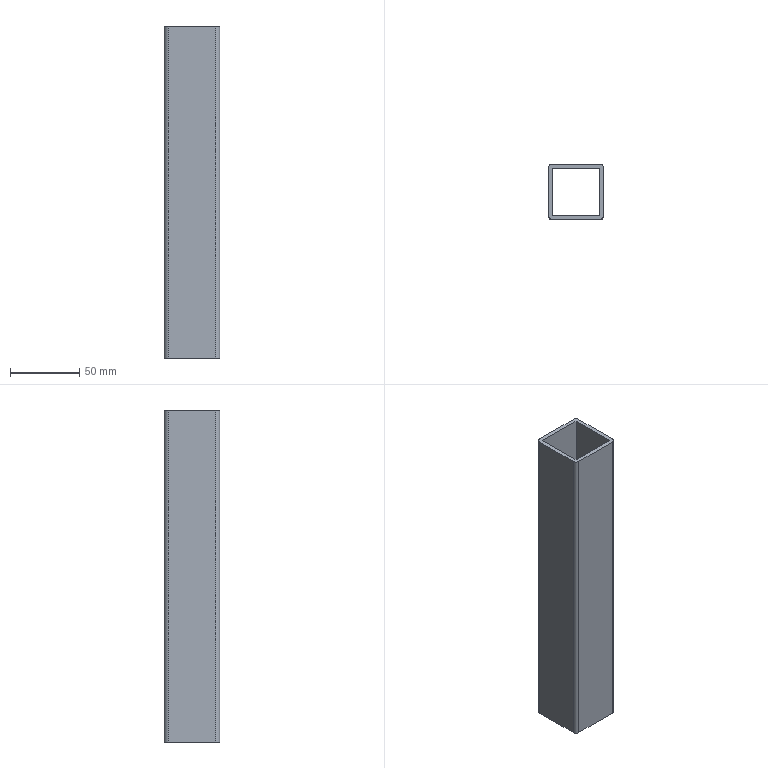Part | STEP file | X77-04203 | 1 solid | 14 faces | box 40 x 40 x 240 mm | volume 104706 mm3 | plane 10 | cylinder 4 | commonest cylinder face diameters 6 x4
STEP:
#1=CARTESIAN_POINT('',(-20.,-17.,240.));
#2=VERTEX_POINT('',#1);
#3=CARTESIAN_POINT('',(-17.,-20.,240.));
#4=VERTEX_POINT('',#3);
#5=CARTESIAN_POINT('',(-17.,-17.,240.));
#6=DIRECTION('',(0.,0.,1.));
#7=DIRECTION('',(-1.,0.,0.));
#8=AXIS2_PLACEMENT_3D('',#5,#6,#7);
#9=CIRCLE('',#8,3.);
#10=EDGE_CURVE('',#2,#4,#9,.T.);
#11=ORIENTED_EDGE('',*,*,#10,.T.);
#12=CARTESIAN_POINT('',(17.,-20.,240.));
#13=VERTEX_POINT('',#12);
#14=CARTESIAN_POINT('',(-17.,-20.,240.));
#15=DIRECTION('',(1.,0.,0.));
#16=VECTOR('',#15,1000.);
#17=LINE('',#14,#16);
#18=EDGE_CURVE('',#4,#13,#17,.T.);
#19=ORIENTED_EDGE('',*,*,#18,.T.);
#20=CARTESIAN_POINT('',(20.,-17.,240.));
#21=VERTEX_POINT('',#20);
#22=CARTESIAN_POINT('',(17.,-17.,240.));
#23=DIRECTION('',(0.,0.,1.));
#24=DIRECTION('',(-1.,0.,0.));
#25=AXIS2_PLACEMENT_3D('',#22,#23,#24);
#26=CIRCLE('',#25,3.);
#27=EDGE_CURVE('',#13,#21,#26,.T.);
#28=ORIENTED_EDGE('',*,*,#27,.T.);
#29=CARTESIAN_POINT('',(20.,17.,240.));
#30=VERTEX_POINT('',#29);
#31=CARTESIAN_POINT('',(20.,-17.,240.));
#32=DIRECTION('',(0.,1.,0.));
#33=VECTOR('',#32,1000.);
#34=LINE('',#31,#33);
#35=EDGE_CURVE('',#21,#30,#34,.T.);
#36=ORIENTED_EDGE('',*,*,#35,.T.);
#37=CARTESIAN_POINT('',(17.,20.,240.));
#38=VERTEX_POINT('',#37);
#39=CARTESIAN_POINT('',(17.,17.,240.));
#40=DIRECTION('',(0.,0.,1.));
#41=DIRECTION('',(1.,0.,0.));
#42=AXIS2_PLACEMENT_3D('',#39,#40,#41);
#43=CIRCLE('',#42,3.);
#44=EDGE_CURVE('',#30,#38,#43,.T.);
#45=ORIENTED_EDGE('',*,*,#44,.T.);
#46=CARTESIAN_POINT('',(-17.,20.,240.));
#47=VERTEX_POINT('',#46);
#48=CARTESIAN_POINT('',(-17.,20.,240.));
#49=DIRECTION('',(-1.,0.,0.));
#50=VECTOR('',#49,1000.);
#51=LINE('',#48,#50);
#52=EDGE_CURVE('',#38,#47,#51,.T.);
#53=ORIENTED_EDGE('',*,*,#52,.T.);
#54=CARTESIAN_POINT('',(-20.,17.,240.));
#55=VERTEX_POINT('',#54);
#56=CARTESIAN_POINT('',(-17.,17.,240.));
#57=DIRECTION('',(0.,0.,1.));
#58=DIRECTION('',(1.,0.,0.));
#59=AXIS2_PLACEMENT_3D('',#56,#57,#58);
#60=CIRCLE('',#59,3.);
#61=EDGE_CURVE('',#47,#55,#60,.T.);
#62=ORIENTED_EDGE('',*,*,#61,.T.);
#63=CARTESIAN_POINT('',(-20.,-17.,240.));
#64=DIRECTION('',(0.,-1.,0.));
#65=VECTOR('',#64,1000.);
#66=LINE('',#63,#65);
#67=EDGE_CURVE('',#55,#2,#66,.T.);
#68=ORIENTED_EDGE('',*,*,#67,.T.);
#69=EDGE_LOOP('',(#11,#19,#28,#36,#45,#53,#62,#68));
#70=FACE_OUTER_BOUND('',#69,.T.);
#71=CARTESIAN_POINT('',(17.,-17.,240.));
#72=VERTEX_POINT('',#71);
#73=CARTESIAN_POINT('',(17.,17.,240.));
#74=VERTEX_POINT('',#73);
#75=CARTESIAN_POINT('',(17.,-17.,240.));
#76=DIRECTION('',(0.,1.,0.));
#77=VECTOR('',#76,1000.);
#78=LINE('',#75,#77);
#79=EDGE_CURVE('',#72,#74,#78,.T.);
#80=ORIENTED_EDGE('',*,*,#79,.F.);
#81=CARTESIAN_POINT('',(-17.,-17.,240.));
#82=VERTEX_POINT('',#81);
#83=CARTESIAN_POINT('',(-17.,-17.,240.));
#84=DIRECTION('',(1.,0.,0.));
#85=VECTOR('',#84,1000.);
#86=LINE('',#83,#85);
#87=EDGE_CURVE('',#82,#72,#86,.T.);
#88=ORIENTED_EDGE('',*,*,#87,.F.);
#89=CARTESIAN_POINT('',(-17.,17.,240.));
#90=VERTEX_POINT('',#89);
#91=CARTESIAN_POINT('',(-17.,-17.,240.));
#92=DIRECTION('',(0.,-1.,0.));
#93=VECTOR('',#92,1000.);
#94=LINE('',#91,#93);
#95=EDGE_CURVE('',#90,#82,#94,.T.);
#96=ORIENTED_EDGE('',*,*,#95,.F.);
#97=CARTESIAN_POINT('',(-17.,17.,240.));
#98=DIRECTION('',(-1.,0.,0.));
#99=VECTOR('',#98,1000.);
#100=LINE('',#97,#99);
#101=EDGE_CURVE('',#74,#90,#100,.T.);
#102=ORIENTED_EDGE('',*,*,#101,.F.);
#103=EDGE_LOOP('',(#80,#88,#96,#102));
#104=FACE_BOUND('',#103,.T.);
#105=CARTESIAN_POINT('',(-17.,-17.,240.));
#106=DIRECTION('',(0.,0.,-1.));
#107=DIRECTION('',(-1.,0.,0.));
#108=AXIS2_PLACEMENT_3D('',#105,#106,#107);
#109=PLANE('',#108);
#110=ADVANCED_FACE('',(#70,#104),#109,.F.);
#111=CARTESIAN_POINT('',(-20.,-17.,0.));
#112=VERTEX_POINT('',#111);
#113=CARTESIAN_POINT('',(-17.,-20.,0.));
#114=VERTEX_POINT('',#113);
#115=CARTESIAN_POINT('',(-17.,-17.,0.));
#116=DIRECTION('',(0.,0.,1.));
#117=DIRECTION('',(-1.,0.,0.));
#118=AXIS2_PLACEMENT_3D('',#115,#116,#117);
#119=CIRCLE('',#118,3.);
#120=EDGE_CURVE('',#112,#114,#119,.T.);
#121=ORIENTED_EDGE('',*,*,#120,.F.);
#122=CARTESIAN_POINT('',(-20.,17.,0.));
#123=VERTEX_POINT('',#122);
#124=CARTESIAN_POINT('',(-20.,-17.,0.));
#125=DIRECTION('',(0.,-1.,0.));
#126=VECTOR('',#125,1000.);
#127=LINE('',#124,#126);
#128=EDGE_CURVE('',#123,#112,#127,.T.);
#129=ORIENTED_EDGE('',*,*,#128,.F.);
#130=CARTESIAN_POINT('',(-17.,20.,0.));
#131=VERTEX_POINT('',#130);
#132=CARTESIAN_POINT('',(-17.,17.,0.));
#133=DIRECTION('',(0.,0.,1.));
#134=DIRECTION('',(1.,0.,0.));
#135=AXIS2_PLACEMENT_3D('',#132,#133,#134);
#136=CIRCLE('',#135,3.);
#137=EDGE_CURVE('',#131,#123,#136,.T.);
#138=ORIENTED_EDGE('',*,*,#137,.F.);
#139=CARTESIAN_POINT('',(17.,20.,0.));
#140=VERTEX_POINT('',#139);
#141=CARTESIAN_POINT('',(-17.,20.,0.));
#142=DIRECTION('',(-1.,0.,0.));
#143=VECTOR('',#142,1000.);
#144=LINE('',#141,#143);
#145=EDGE_CURVE('',#140,#131,#144,.T.);
#146=ORIENTED_EDGE('',*,*,#145,.F.);
#147=CARTESIAN_POINT('',(20.,17.,0.));
#148=VERTEX_POINT('',#147);
#149=CARTESIAN_POINT('',(17.,17.,0.));
#150=DIRECTION('',(0.,0.,1.));
#151=DIRECTION('',(1.,0.,0.));
#152=AXIS2_PLACEMENT_3D('',#149,#150,#151);
#153=CIRCLE('',#152,3.);
#154=EDGE_CURVE('',#148,#140,#153,.T.);
#155=ORIENTED_EDGE('',*,*,#154,.F.);
#156=CARTESIAN_POINT('',(20.,-17.,0.));
#157=VERTEX_POINT('',#156);
#158=CARTESIAN_POINT('',(20.,-17.,0.));
#159=DIRECTION('',(0.,1.,0.));
#160=VECTOR('',#159,1000.);
#161=LINE('',#158,#160);
#162=EDGE_CURVE('',#157,#148,#161,.T.);
#163=ORIENTED_EDGE('',*,*,#162,.F.);
#164=CARTESIAN_POINT('',(17.,-20.,0.));
#165=VERTEX_POINT('',#164);
#166=CARTESIAN_POINT('',(17.,-17.,0.));
#167=DIRECTION('',(0.,0.,1.));
#168=DIRECTION('',(-1.,0.,0.));
#169=AXIS2_PLACEMENT_3D('',#166,#167,#168);
#170=CIRCLE('',#169,3.);
#171=EDGE_CURVE('',#165,#157,#170,.T.);
#172=ORIENTED_EDGE('',*,*,#171,.F.);
#173=CARTESIAN_POINT('',(-17.,-20.,0.));
#174=DIRECTION('',(1.,0.,0.));
#175=VECTOR('',#174,1000.);
#176=LINE('',#173,#175);
#177=EDGE_CURVE('',#114,#165,#176,.T.);
#178=ORIENTED_EDGE('',*,*,#177,.F.);
#179=EDGE_LOOP('',(#121,#129,#138,#146,#155,#163,#172,#178));
#180=FACE_OUTER_BOUND('',#179,.T.);
#181=CARTESIAN_POINT('',(-17.,-17.,0.));
#182=VERTEX_POINT('',#181);
#183=CARTESIAN_POINT('',(17.,-17.,0.));
#184=VERTEX_POINT('',#183);
#185=CARTESIAN_POINT('',(-17.,-17.,0.));
#186=DIRECTION('',(1.,0.,0.));
#187=VECTOR('',#186,1000.);
#188=LINE('',#185,#187);
#189=EDGE_CURVE('',#182,#184,#188,.T.);
#190=ORIENTED_EDGE('',*,*,#189,.T.);
#191=CARTESIAN_POINT('',(17.,17.,0.));
#192=VERTEX_POINT('',#191);
#193=CARTESIAN_POINT('',(17.,-17.,0.));
#194=DIRECTION('',(0.,1.,0.));
#195=VECTOR('',#194,1000.);
#196=LINE('',#193,#195);
#197=EDGE_CURVE('',#184,#192,#196,.T.);
#198=ORIENTED_EDGE('',*,*,#197,.T.);
#199=CARTESIAN_POINT('',(-17.,17.,0.));
#200=VERTEX_POINT('',#199);
#201=CARTESIAN_POINT('',(-17.,17.,0.));
#202=DIRECTION('',(-1.,0.,0.));
#203=VECTOR('',#202,1000.);
#204=LINE('',#201,#203);
#205=EDGE_CURVE('',#192,#200,#204,.T.);
#206=ORIENTED_EDGE('',*,*,#205,.T.);
#207=CARTESIAN_POINT('',(-17.,-17.,0.));
#208=DIRECTION('',(0.,-1.,0.));
#209=VECTOR('',#208,1000.);
#210=LINE('',#207,#209);
#211=EDGE_CURVE('',#200,#182,#210,.T.);
#212=ORIENTED_EDGE('',*,*,#211,.T.);
#213=EDGE_LOOP('',(#190,#198,#206,#212));
#214=FACE_BOUND('',#213,.T.);
#215=CARTESIAN_POINT('',(-17.,-17.,0.));
#216=DIRECTION('',(0.,0.,-1.));
#217=DIRECTION('',(-1.,0.,0.));
#218=AXIS2_PLACEMENT_3D('',#215,#216,#217);
#219=PLANE('',#218);
#220=ADVANCED_FACE('',(#180,#214),#219,.T.);
#221=ORIENTED_EDGE('',*,*,#120,.T.);
#222=CARTESIAN_POINT('',(-17.,-20.,240.));
#223=DIRECTION('',(0.,0.,-1.));
#224=VECTOR('',#223,1000.);
#225=LINE('',#222,#224);
#226=EDGE_CURVE('',#4,#114,#225,.T.);
#227=ORIENTED_EDGE('',*,*,#226,.F.);
#228=ORIENTED_EDGE('',*,*,#10,.F.);
#229=CARTESIAN_POINT('',(-20.,-17.,240.));
#230=DIRECTION('',(0.,0.,-1.));
#231=VECTOR('',#230,1000.);
#232=LINE('',#229,#231);
#233=EDGE_CURVE('',#2,#112,#232,.T.);
#234=ORIENTED_EDGE('',*,*,#233,.T.);
#235=EDGE_LOOP('',(#221,#227,#228,#234));
#236=FACE_OUTER_BOUND('',#235,.T.);
#237=CARTESIAN_POINT('',(-17.,-17.,240.));
#238=DIRECTION('',(0.,0.,-1.));
#239=DIRECTION('',(-1.,0.,0.));
#240=AXIS2_PLACEMENT_3D('',#237,#238,#239);
#241=CYLINDRICAL_SURFACE('',#240,3.);
#242=ADVANCED_FACE('',(#236),#241,.T.);
#243=ORIENTED_EDGE('',*,*,#177,.T.);
#244=CARTESIAN_POINT('',(17.,-20.,240.));
#245=DIRECTION('',(0.,0.,-1.));
#246=VECTOR('',#245,1000.);
#247=LINE('',#244,#246);
#248=EDGE_CURVE('',#13,#165,#247,.T.);
#249=ORIENTED_EDGE('',*,*,#248,.F.);
#250=ORIENTED_EDGE('',*,*,#18,.F.);
#251=ORIENTED_EDGE('',*,*,#226,.T.);
#252=EDGE_LOOP('',(#243,#249,#250,#251));
#253=FACE_OUTER_BOUND('',#252,.T.);
#254=CARTESIAN_POINT('',(-17.,-20.,240.));
#255=DIRECTION('',(0.,1.,0.));
#256=DIRECTION('',(0.,0.,1.));
#257=AXIS2_PLACEMENT_3D('',#254,#255,#256);
#258=PLANE('',#257);
#259=ADVANCED_FACE('',(#253),#258,.F.);
#260=ORIENTED_EDGE('',*,*,#171,.T.);
#261=CARTESIAN_POINT('',(20.,-17.,240.));
#262=DIRECTION('',(0.,0.,-1.));
#263=VECTOR('',#262,1000.);
#264=LINE('',#261,#263);
#265=EDGE_CURVE('',#21,#157,#264,.T.);
#266=ORIENTED_EDGE('',*,*,#265,.F.);
#267=ORIENTED_EDGE('',*,*,#27,.F.);
#268=ORIENTED_EDGE('',*,*,#248,.T.);
#269=EDGE_LOOP('',(#260,#266,#267,#268));
#270=FACE_OUTER_BOUND('',#269,.T.);
#271=CARTESIAN_POINT('',(17.,-17.,240.));
#272=DIRECTION('',(0.,0.,-1.));
#273=DIRECTION('',(-1.,0.,0.));
#274=AXIS2_PLACEMENT_3D('',#271,#272,#273);
#275=CYLINDRICAL_SURFACE('',#274,3.);
#276=ADVANCED_FACE('',(#270),#275,.T.);
#277=ORIENTED_EDGE('',*,*,#162,.T.);
#278=CARTESIAN_POINT('',(20.,17.,240.));
#279=DIRECTION('',(0.,0.,-1.));
#280=VECTOR('',#279,1000.);
#281=LINE('',#278,#280);
#282=EDGE_CURVE('',#30,#148,#281,.T.);
#283=ORIENTED_EDGE('',*,*,#282,.F.);
#284=ORIENTED_EDGE('',*,*,#35,.F.);
#285=ORIENTED_EDGE('',*,*,#265,.T.);
#286=EDGE_LOOP('',(#277,#283,#284,#285));
#287=FACE_OUTER_BOUND('',#286,.T.);
#288=CARTESIAN_POINT('',(20.,-17.,240.));
#289=DIRECTION('',(-1.,0.,0.));
#290=DIRECTION('',(0.,0.,1.));
#291=AXIS2_PLACEMENT_3D('',#288,#289,#290);
#292=PLANE('',#291);
#293=ADVANCED_FACE('',(#287),#292,.F.);
#294=ORIENTED_EDGE('',*,*,#154,.T.);
#295=CARTESIAN_POINT('',(17.,20.,240.));
#296=DIRECTION('',(0.,0.,-1.));
#297=VECTOR('',#296,1000.);
#298=LINE('',#295,#297);
#299=EDGE_CURVE('',#38,#140,#298,.T.);
#300=ORIENTED_EDGE('',*,*,#299,.F.);
#301=ORIENTED_EDGE('',*,*,#44,.F.);
#302=ORIENTED_EDGE('',*,*,#282,.T.);
#303=EDGE_LOOP('',(#294,#300,#301,#302));
#304=FACE_OUTER_BOUND('',#303,.T.);
#305=CARTESIAN_POINT('',(17.,17.,240.));
#306=DIRECTION('',(0.,0.,-1.));
#307=DIRECTION('',(-1.,0.,0.));
#308=AXIS2_PLACEMENT_3D('',#305,#306,#307);
#309=CYLINDRICAL_SURFACE('',#308,3.);
#310=ADVANCED_FACE('',(#304),#309,.T.);
#311=ORIENTED_EDGE('',*,*,#145,.T.);
#312=CARTESIAN_POINT('',(-17.,20.,240.));
#313=DIRECTION('',(0.,0.,-1.));
#314=VECTOR('',#313,1000.);
#315=LINE('',#312,#314);
#316=EDGE_CURVE('',#47,#131,#315,.T.);
#317=ORIENTED_EDGE('',*,*,#316,.F.);
#318=ORIENTED_EDGE('',*,*,#52,.F.);
#319=ORIENTED_EDGE('',*,*,#299,.T.);
#320=EDGE_LOOP('',(#311,#317,#318,#319));
#321=FACE_OUTER_BOUND('',#320,.T.);
#322=CARTESIAN_POINT('',(-17.,20.,240.));
#323=DIRECTION('',(0.,-1.,0.));
#324=DIRECTION('',(0.,0.,-1.));
#325=AXIS2_PLACEMENT_3D('',#322,#323,#324);
#326=PLANE('',#325);
#327=ADVANCED_FACE('',(#321),#326,.F.);
#328=ORIENTED_EDGE('',*,*,#137,.T.);
#329=CARTESIAN_POINT('',(-20.,17.,240.));
#330=DIRECTION('',(0.,0.,-1.));
#331=VECTOR('',#330,1000.);
#332=LINE('',#329,#331);
#333=EDGE_CURVE('',#55,#123,#332,.T.);
#334=ORIENTED_EDGE('',*,*,#333,.F.);
#335=ORIENTED_EDGE('',*,*,#61,.F.);
#336=ORIENTED_EDGE('',*,*,#316,.T.);
#337=EDGE_LOOP('',(#328,#334,#335,#336));
#338=FACE_OUTER_BOUND('',#337,.T.);
#339=CARTESIAN_POINT('',(-17.,17.,240.));
#340=DIRECTION('',(0.,0.,-1.));
#341=DIRECTION('',(-1.,0.,0.));
#342=AXIS2_PLACEMENT_3D('',#339,#340,#341);
#343=CYLINDRICAL_SURFACE('',#342,3.);
#344=ADVANCED_FACE('',(#338),#343,.T.);
#345=ORIENTED_EDGE('',*,*,#128,.T.);
#346=ORIENTED_EDGE('',*,*,#233,.F.);
#347=ORIENTED_EDGE('',*,*,#67,.F.);
#348=ORIENTED_EDGE('',*,*,#333,.T.);
#349=EDGE_LOOP('',(#345,#346,#347,#348));
#350=FACE_OUTER_BOUND('',#349,.T.);
#351=CARTESIAN_POINT('',(-20.,-17.,240.));
#352=DIRECTION('',(1.,0.,0.));
#353=DIRECTION('',(0.,0.,-1.));
#354=AXIS2_PLACEMENT_3D('',#351,#352,#353);
#355=PLANE('',#354);
#356=ADVANCED_FACE('',(#350),#355,.F.);
#357=ORIENTED_EDGE('',*,*,#197,.F.);
#358=CARTESIAN_POINT('',(17.,-17.,240.));
#359=DIRECTION('',(0.,0.,-1.));
#360=VECTOR('',#359,1000.);
#361=LINE('',#358,#360);
#362=EDGE_CURVE('',#72,#184,#361,.T.);
#363=ORIENTED_EDGE('',*,*,#362,.F.);
#364=ORIENTED_EDGE('',*,*,#79,.T.);
#365=CARTESIAN_POINT('',(17.,17.,240.));
#366=DIRECTION('',(0.,0.,-1.));
#367=VECTOR('',#366,1000.);
#368=LINE('',#365,#367);
#369=EDGE_CURVE('',#74,#192,#368,.T.);
#370=ORIENTED_EDGE('',*,*,#369,.T.);
#371=EDGE_LOOP('',(#357,#363,#364,#370));
#372=FACE_OUTER_BOUND('',#371,.T.);
#373=CARTESIAN_POINT('',(17.,-17.,240.));
#374=DIRECTION('',(-1.,0.,0.));
#375=DIRECTION('',(0.,0.,1.));
#376=AXIS2_PLACEMENT_3D('',#373,#374,#375);
#377=PLANE('',#376);
#378=ADVANCED_FACE('',(#372),#377,.T.);
#379=ORIENTED_EDGE('',*,*,#205,.F.);
#380=ORIENTED_EDGE('',*,*,#369,.F.);
#381=ORIENTED_EDGE('',*,*,#101,.T.);
#382=CARTESIAN_POINT('',(-17.,17.,240.));
#383=DIRECTION('',(0.,0.,-1.));
#384=VECTOR('',#383,1000.);
#385=LINE('',#382,#384);
#386=EDGE_CURVE('',#90,#200,#385,.T.);
#387=ORIENTED_EDGE('',*,*,#386,.T.);
#388=EDGE_LOOP('',(#379,#380,#381,#387));
#389=FACE_OUTER_BOUND('',#388,.T.);
#390=CARTESIAN_POINT('',(-17.,17.,240.));
#391=DIRECTION('',(0.,-1.,0.));
#392=DIRECTION('',(0.,0.,-1.));
#393=AXIS2_PLACEMENT_3D('',#390,#391,#392);
#394=PLANE('',#393);
#395=ADVANCED_FACE('',(#389),#394,.T.);
#396=ORIENTED_EDGE('',*,*,#211,.F.);
#397=ORIENTED_EDGE('',*,*,#386,.F.);
#398=ORIENTED_EDGE('',*,*,#95,.T.);
#399=CARTESIAN_POINT('',(-17.,-17.,240.));
#400=DIRECTION('',(0.,0.,-1.));
#401=VECTOR('',#400,1000.);
#402=LINE('',#399,#401);
#403=EDGE_CURVE('',#82,#182,#402,.T.);
#404=ORIENTED_EDGE('',*,*,#403,.T.);
#405=EDGE_LOOP('',(#396,#397,#398,#404));
#406=FACE_OUTER_BOUND('',#405,.T.);
#407=CARTESIAN_POINT('',(-17.,-17.,240.));
#408=DIRECTION('',(1.,0.,0.));
#409=DIRECTION('',(0.,0.,-1.));
#410=AXIS2_PLACEMENT_3D('',#407,#408,#409);
#411=PLANE('',#410);
#412=ADVANCED_FACE('',(#406),#411,.T.);
#413=ORIENTED_EDGE('',*,*,#189,.F.);
#414=ORIENTED_EDGE('',*,*,#403,.F.);
#415=ORIENTED_EDGE('',*,*,#87,.T.);
#416=ORIENTED_EDGE('',*,*,#362,.T.);
#417=EDGE_LOOP('',(#413,#414,#415,#416));
#418=FACE_OUTER_BOUND('',#417,.T.);
#419=CARTESIAN_POINT('',(-17.,-17.,240.));
#420=DIRECTION('',(0.,1.,0.));
#421=DIRECTION('',(0.,0.,1.));
#422=AXIS2_PLACEMENT_3D('',#419,#420,#421);
#423=PLANE('',#422);
#424=ADVANCED_FACE('',(#418),#423,.T.);
#425=CLOSED_SHELL('',(#110,#220,#242,#259,#276,#293,#310,#327,#344,#356,#378,#395,#412,#424));
#426=MANIFOLD_SOLID_BREP('',#425);
#427=CARTESIAN_POINT('',(0.,0.,0.));
#428=DIRECTION('',(0.,0.,1.));
#429=DIRECTION('',(1.,0.,0.));
#430=AXIS2_PLACEMENT_3D('',#427,#428,#429);
#431=(LENGTH_UNIT()NAMED_UNIT(*)SI_UNIT(.MILLI.,.METRE.));
#432=UNCERTAINTY_MEASURE_WITH_UNIT(LENGTH_MEASURE(0.00001),#431,'','');
#433=(NAMED_UNIT(*)PLANE_ANGLE_UNIT()SI_UNIT($,.RADIAN.));
#434=(NAMED_UNIT(*)SI_UNIT($,.STERADIAN.)SOLID_ANGLE_UNIT());
#435=(GEOMETRIC_REPRESENTATION_CONTEXT(3)GLOBAL_UNCERTAINTY_ASSIGNED_CONTEXT((#432))GLOBAL_UNIT_ASSIGNED_CONTEXT((#431,#433,#434))REPRESENTATION_CONTEXT('',''));
#436=ADVANCED_BREP_SHAPE_REPRESENTATION('',(#426,#430),#435);